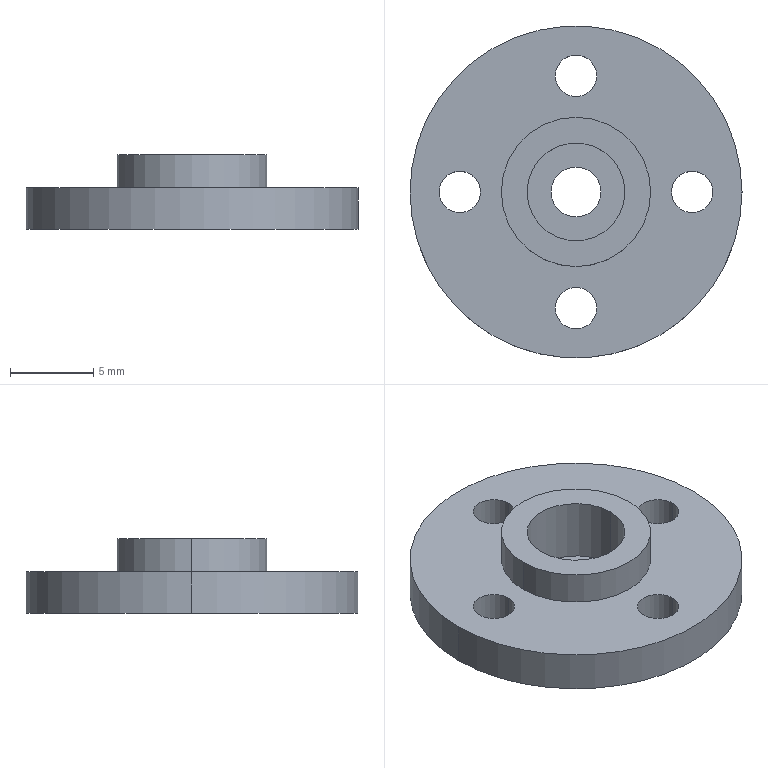Part | SolidWorks | features ICE 4, Extrusion 1, HoleWzd 1 | 1 solid | 20 faces | box 20 x 20 x 4.5 mm | volume 753.693 mm3 | cylinder 16 | plane 4 | commonest cylinder face diameters 2.5 x8 3 x2 5.9 x2 9 x2 20 x2
STEP:
#1=CARTESIAN_POINT('',(-8.25,0.,0.));
#2=VERTEX_POINT('',#1);
#3=CARTESIAN_POINT('',(-5.75,0.,0.));
#4=VERTEX_POINT('',#3);
#5=CARTESIAN_POINT('',(-7.,0.,0.));
#6=DIRECTION('',(0.,0.,1.));
#7=DIRECTION('',(1.,0.,0.));
#8=AXIS2_PLACEMENT_3D('',#5,#6,#7);
#9=CIRCLE('',#8,1.25);
#10=EDGE_CURVE('',#2,#4,#9,.T.);
#11=ORIENTED_EDGE('',*,*,#10,.F.);
#12=CARTESIAN_POINT('',(-8.25,0.,2.5));
#13=VERTEX_POINT('',#12);
#14=CARTESIAN_POINT('',(-8.25,0.,2.5));
#15=DIRECTION('',(0.,0.,1.));
#16=VECTOR('',#15,1000.);
#17=LINE('',#14,#16);
#18=EDGE_CURVE('',#2,#13,#17,.T.);
#19=ORIENTED_EDGE('',*,*,#18,.T.);
#20=CARTESIAN_POINT('',(-5.75,0.,2.5));
#21=VERTEX_POINT('',#20);
#22=CARTESIAN_POINT('',(-7.,0.,2.5));
#23=DIRECTION('',(0.,0.,1.));
#24=DIRECTION('',(1.,0.,0.));
#25=AXIS2_PLACEMENT_3D('',#22,#23,#24);
#26=CIRCLE('',#25,1.25);
#27=EDGE_CURVE('',#13,#21,#26,.T.);
#28=ORIENTED_EDGE('',*,*,#27,.T.);
#29=CARTESIAN_POINT('',(-5.75,0.,2.5));
#30=DIRECTION('',(0.,0.,1.));
#31=VECTOR('',#30,1000.);
#32=LINE('',#29,#31);
#33=EDGE_CURVE('',#4,#21,#32,.T.);
#34=ORIENTED_EDGE('',*,*,#33,.F.);
#35=EDGE_LOOP('',(#11,#19,#28,#34));
#36=FACE_OUTER_BOUND('',#35,.T.);
#37=CARTESIAN_POINT('',(-7.,0.,2.5));
#38=DIRECTION('',(0.,0.,1.));
#39=DIRECTION('',(1.,0.,0.));
#40=AXIS2_PLACEMENT_3D('',#37,#38,#39);
#41=CYLINDRICAL_SURFACE('',#40,1.25);
#42=ADVANCED_FACE('',(#36),#41,.F.);
#43=CARTESIAN_POINT('',(-1.25,7.,0.));
#44=VERTEX_POINT('',#43);
#45=CARTESIAN_POINT('',(1.25,7.,0.));
#46=VERTEX_POINT('',#45);
#47=CARTESIAN_POINT('',(0.,7.,0.));
#48=DIRECTION('',(0.,0.,1.));
#49=DIRECTION('',(1.,0.,0.));
#50=AXIS2_PLACEMENT_3D('',#47,#48,#49);
#51=CIRCLE('',#50,1.25);
#52=EDGE_CURVE('',#44,#46,#51,.T.);
#53=ORIENTED_EDGE('',*,*,#52,.F.);
#54=CARTESIAN_POINT('',(-1.25,7.,2.5));
#55=VERTEX_POINT('',#54);
#56=CARTESIAN_POINT('',(-1.25,7.,2.5));
#57=DIRECTION('',(0.,0.,1.));
#58=VECTOR('',#57,1000.);
#59=LINE('',#56,#58);
#60=EDGE_CURVE('',#44,#55,#59,.T.);
#61=ORIENTED_EDGE('',*,*,#60,.T.);
#62=CARTESIAN_POINT('',(1.25,7.,2.5));
#63=VERTEX_POINT('',#62);
#64=CARTESIAN_POINT('',(0.,7.,2.5));
#65=DIRECTION('',(0.,0.,1.));
#66=DIRECTION('',(1.,0.,0.));
#67=AXIS2_PLACEMENT_3D('',#64,#65,#66);
#68=CIRCLE('',#67,1.25);
#69=EDGE_CURVE('',#55,#63,#68,.T.);
#70=ORIENTED_EDGE('',*,*,#69,.T.);
#71=CARTESIAN_POINT('',(1.25,7.,2.5));
#72=DIRECTION('',(0.,0.,1.));
#73=VECTOR('',#72,1000.);
#74=LINE('',#71,#73);
#75=EDGE_CURVE('',#46,#63,#74,.T.);
#76=ORIENTED_EDGE('',*,*,#75,.F.);
#77=EDGE_LOOP('',(#53,#61,#70,#76));
#78=FACE_OUTER_BOUND('',#77,.T.);
#79=CARTESIAN_POINT('',(0.,7.,2.5));
#80=DIRECTION('',(0.,0.,1.));
#81=DIRECTION('',(1.,0.,0.));
#82=AXIS2_PLACEMENT_3D('',#79,#80,#81);
#83=CYLINDRICAL_SURFACE('',#82,1.25);
#84=ADVANCED_FACE('',(#78),#83,.F.);
#85=CARTESIAN_POINT('',(5.75,0.,0.));
#86=VERTEX_POINT('',#85);
#87=CARTESIAN_POINT('',(8.25,0.,0.));
#88=VERTEX_POINT('',#87);
#89=CARTESIAN_POINT('',(7.,0.,0.));
#90=DIRECTION('',(0.,0.,1.));
#91=DIRECTION('',(1.,0.,0.));
#92=AXIS2_PLACEMENT_3D('',#89,#90,#91);
#93=CIRCLE('',#92,1.25);
#94=EDGE_CURVE('',#86,#88,#93,.T.);
#95=ORIENTED_EDGE('',*,*,#94,.F.);
#96=CARTESIAN_POINT('',(5.75,0.,2.5));
#97=VERTEX_POINT('',#96);
#98=CARTESIAN_POINT('',(5.75,0.,2.5));
#99=DIRECTION('',(0.,0.,1.));
#100=VECTOR('',#99,1000.);
#101=LINE('',#98,#100);
#102=EDGE_CURVE('',#86,#97,#101,.T.);
#103=ORIENTED_EDGE('',*,*,#102,.T.);
#104=CARTESIAN_POINT('',(8.25,0.,2.5));
#105=VERTEX_POINT('',#104);
#106=CARTESIAN_POINT('',(7.,0.,2.5));
#107=DIRECTION('',(0.,0.,1.));
#108=DIRECTION('',(1.,0.,0.));
#109=AXIS2_PLACEMENT_3D('',#106,#107,#108);
#110=CIRCLE('',#109,1.25);
#111=EDGE_CURVE('',#97,#105,#110,.T.);
#112=ORIENTED_EDGE('',*,*,#111,.T.);
#113=CARTESIAN_POINT('',(8.25,0.,2.5));
#114=DIRECTION('',(0.,0.,1.));
#115=VECTOR('',#114,1000.);
#116=LINE('',#113,#115);
#117=EDGE_CURVE('',#88,#105,#116,.T.);
#118=ORIENTED_EDGE('',*,*,#117,.F.);
#119=EDGE_LOOP('',(#95,#103,#112,#118));
#120=FACE_OUTER_BOUND('',#119,.T.);
#121=CARTESIAN_POINT('',(7.,0.,2.5));
#122=DIRECTION('',(0.,0.,1.));
#123=DIRECTION('',(1.,0.,0.));
#124=AXIS2_PLACEMENT_3D('',#121,#122,#123);
#125=CYLINDRICAL_SURFACE('',#124,1.25);
#126=ADVANCED_FACE('',(#120),#125,.F.);
#127=CARTESIAN_POINT('',(-1.25,-7.,0.));
#128=VERTEX_POINT('',#127);
#129=CARTESIAN_POINT('',(1.25,-7.,0.));
#130=VERTEX_POINT('',#129);
#131=CARTESIAN_POINT('',(0.,-7.,0.));
#132=DIRECTION('',(0.,0.,1.));
#133=DIRECTION('',(1.,0.,0.));
#134=AXIS2_PLACEMENT_3D('',#131,#132,#133);
#135=CIRCLE('',#134,1.25);
#136=EDGE_CURVE('',#128,#130,#135,.T.);
#137=ORIENTED_EDGE('',*,*,#136,.F.);
#138=CARTESIAN_POINT('',(-1.25,-7.,2.5));
#139=VERTEX_POINT('',#138);
#140=CARTESIAN_POINT('',(-1.25,-7.,2.5));
#141=DIRECTION('',(0.,0.,1.));
#142=VECTOR('',#141,1000.);
#143=LINE('',#140,#142);
#144=EDGE_CURVE('',#128,#139,#143,.T.);
#145=ORIENTED_EDGE('',*,*,#144,.T.);
#146=CARTESIAN_POINT('',(1.25,-7.,2.5));
#147=VERTEX_POINT('',#146);
#148=CARTESIAN_POINT('',(0.,-7.,2.5));
#149=DIRECTION('',(0.,0.,1.));
#150=DIRECTION('',(1.,0.,0.));
#151=AXIS2_PLACEMENT_3D('',#148,#149,#150);
#152=CIRCLE('',#151,1.25);
#153=EDGE_CURVE('',#139,#147,#152,.T.);
#154=ORIENTED_EDGE('',*,*,#153,.T.);
#155=CARTESIAN_POINT('',(1.25,-7.,2.5));
#156=DIRECTION('',(0.,0.,1.));
#157=VECTOR('',#156,1000.);
#158=LINE('',#155,#157);
#159=EDGE_CURVE('',#130,#147,#158,.T.);
#160=ORIENTED_EDGE('',*,*,#159,.F.);
#161=EDGE_LOOP('',(#137,#145,#154,#160));
#162=FACE_OUTER_BOUND('',#161,.T.);
#163=CARTESIAN_POINT('',(0.,-7.,2.5));
#164=DIRECTION('',(0.,0.,1.));
#165=DIRECTION('',(1.,0.,0.));
#166=AXIS2_PLACEMENT_3D('',#163,#164,#165);
#167=CYLINDRICAL_SURFACE('',#166,1.25);
#168=ADVANCED_FACE('',(#162),#167,.F.);
#169=CARTESIAN_POINT('',(-1.5,0.,0.));
#170=VERTEX_POINT('',#169);
#171=CARTESIAN_POINT('',(1.5,0.,0.));
#172=VERTEX_POINT('',#171);
#173=CARTESIAN_POINT('',(0.,0.,0.));
#174=DIRECTION('',(0.,0.,1.));
#175=DIRECTION('',(1.,0.,0.));
#176=AXIS2_PLACEMENT_3D('',#173,#174,#175);
#177=CIRCLE('',#176,1.5);
#178=EDGE_CURVE('',#170,#172,#177,.T.);
#179=ORIENTED_EDGE('',*,*,#178,.F.);
#180=CARTESIAN_POINT('',(-1.5,0.,0.65));
#181=VERTEX_POINT('',#180);
#182=CARTESIAN_POINT('',(-1.5,0.,0.));
#183=DIRECTION('',(0.,0.,1.));
#184=VECTOR('',#183,1000.);
#185=LINE('',#182,#184);
#186=EDGE_CURVE('',#170,#181,#185,.T.);
#187=ORIENTED_EDGE('',*,*,#186,.T.);
#188=CARTESIAN_POINT('',(1.5,0.,0.65));
#189=VERTEX_POINT('',#188);
#190=CARTESIAN_POINT('',(0.,0.,0.65));
#191=DIRECTION('',(0.,0.,1.));
#192=DIRECTION('',(1.,0.,0.));
#193=AXIS2_PLACEMENT_3D('',#190,#191,#192);
#194=CIRCLE('',#193,1.5);
#195=EDGE_CURVE('',#181,#189,#194,.T.);
#196=ORIENTED_EDGE('',*,*,#195,.T.);
#197=CARTESIAN_POINT('',(1.5,0.,0.));
#198=DIRECTION('',(0.,0.,1.));
#199=VECTOR('',#198,1000.);
#200=LINE('',#197,#199);
#201=EDGE_CURVE('',#172,#189,#200,.T.);
#202=ORIENTED_EDGE('',*,*,#201,.F.);
#203=EDGE_LOOP('',(#179,#187,#196,#202));
#204=FACE_OUTER_BOUND('',#203,.T.);
#205=CARTESIAN_POINT('',(0.,0.,0.));
#206=DIRECTION('',(0.,0.,1.));
#207=DIRECTION('',(1.,0.,0.));
#208=AXIS2_PLACEMENT_3D('',#205,#206,#207);
#209=CYLINDRICAL_SURFACE('',#208,1.5);
#210=ADVANCED_FACE('',(#204),#209,.F.);
#211=CARTESIAN_POINT('',(-2.95,0.,0.65));
#212=VERTEX_POINT('',#211);
#213=CARTESIAN_POINT('',(2.95,0.,0.65));
#214=VERTEX_POINT('',#213);
#215=CARTESIAN_POINT('',(0.,0.,0.65));
#216=DIRECTION('',(0.,0.,1.));
#217=DIRECTION('',(1.,0.,0.));
#218=AXIS2_PLACEMENT_3D('',#215,#216,#217);
#219=CIRCLE('',#218,2.95);
#220=EDGE_CURVE('',#212,#214,#219,.T.);
#221=ORIENTED_EDGE('',*,*,#220,.F.);
#222=CARTESIAN_POINT('',(-2.95,0.,4.5));
#223=VERTEX_POINT('',#222);
#224=CARTESIAN_POINT('',(-2.95,0.,0.65));
#225=DIRECTION('',(0.,0.,1.));
#226=VECTOR('',#225,1000.);
#227=LINE('',#224,#226);
#228=EDGE_CURVE('',#212,#223,#227,.T.);
#229=ORIENTED_EDGE('',*,*,#228,.T.);
#230=CARTESIAN_POINT('',(2.95,0.,4.5));
#231=VERTEX_POINT('',#230);
#232=CARTESIAN_POINT('',(0.,0.,4.5));
#233=DIRECTION('',(0.,0.,1.));
#234=DIRECTION('',(1.,0.,0.));
#235=AXIS2_PLACEMENT_3D('',#232,#233,#234);
#236=CIRCLE('',#235,2.95);
#237=EDGE_CURVE('',#223,#231,#236,.T.);
#238=ORIENTED_EDGE('',*,*,#237,.T.);
#239=CARTESIAN_POINT('',(2.95,0.,0.65));
#240=DIRECTION('',(0.,0.,1.));
#241=VECTOR('',#240,1000.);
#242=LINE('',#239,#241);
#243=EDGE_CURVE('',#214,#231,#242,.T.);
#244=ORIENTED_EDGE('',*,*,#243,.F.);
#245=EDGE_LOOP('',(#221,#229,#238,#244));
#246=FACE_OUTER_BOUND('',#245,.T.);
#247=CARTESIAN_POINT('',(0.,0.,0.65));
#248=DIRECTION('',(0.,0.,1.));
#249=DIRECTION('',(1.,0.,0.));
#250=AXIS2_PLACEMENT_3D('',#247,#248,#249);
#251=CYLINDRICAL_SURFACE('',#250,2.95);
#252=ADVANCED_FACE('',(#246),#251,.F.);
#253=CARTESIAN_POINT('',(4.5,0.,2.5));
#254=VERTEX_POINT('',#253);
#255=CARTESIAN_POINT('',(-4.5,0.,2.5));
#256=VERTEX_POINT('',#255);
#257=CARTESIAN_POINT('',(0.,0.,2.5));
#258=DIRECTION('',(0.,0.,1.));
#259=DIRECTION('',(1.,0.,0.));
#260=AXIS2_PLACEMENT_3D('',#257,#258,#259);
#261=CIRCLE('',#260,4.5);
#262=EDGE_CURVE('',#254,#256,#261,.T.);
#263=ORIENTED_EDGE('',*,*,#262,.T.);
#264=CARTESIAN_POINT('',(-4.5,0.,4.5));
#265=VERTEX_POINT('',#264);
#266=CARTESIAN_POINT('',(-4.5,0.,2.5));
#267=DIRECTION('',(0.,0.,1.));
#268=VECTOR('',#267,1000.);
#269=LINE('',#266,#268);
#270=EDGE_CURVE('',#256,#265,#269,.T.);
#271=ORIENTED_EDGE('',*,*,#270,.T.);
#272=CARTESIAN_POINT('',(4.5,0.,4.5));
#273=VERTEX_POINT('',#272);
#274=CARTESIAN_POINT('',(0.,0.,4.5));
#275=DIRECTION('',(0.,0.,1.));
#276=DIRECTION('',(1.,0.,0.));
#277=AXIS2_PLACEMENT_3D('',#274,#275,#276);
#278=CIRCLE('',#277,4.5);
#279=EDGE_CURVE('',#273,#265,#278,.T.);
#280=ORIENTED_EDGE('',*,*,#279,.F.);
#281=CARTESIAN_POINT('',(4.5,0.,2.5));
#282=DIRECTION('',(0.,0.,1.));
#283=VECTOR('',#282,1000.);
#284=LINE('',#281,#283);
#285=EDGE_CURVE('',#254,#273,#284,.T.);
#286=ORIENTED_EDGE('',*,*,#285,.F.);
#287=EDGE_LOOP('',(#263,#271,#280,#286));
#288=FACE_OUTER_BOUND('',#287,.T.);
#289=CARTESIAN_POINT('',(0.,0.,2.5));
#290=DIRECTION('',(0.,0.,1.));
#291=DIRECTION('',(1.,0.,0.));
#292=AXIS2_PLACEMENT_3D('',#289,#290,#291);
#293=CYLINDRICAL_SURFACE('',#292,4.5);
#294=ADVANCED_FACE('',(#288),#293,.T.);
#295=CARTESIAN_POINT('',(10.,0.,2.5));
#296=VERTEX_POINT('',#295);
#297=CARTESIAN_POINT('',(-10.,0.,2.5));
#298=VERTEX_POINT('',#297);
#299=CARTESIAN_POINT('',(0.,0.,2.5));
#300=DIRECTION('',(0.,0.,1.));
#301=DIRECTION('',(1.,0.,0.));
#302=AXIS2_PLACEMENT_3D('',#299,#300,#301);
#303=CIRCLE('',#302,10.);
#304=EDGE_CURVE('',#296,#298,#303,.T.);
#305=ORIENTED_EDGE('',*,*,#304,.F.);
#306=CARTESIAN_POINT('',(10.,0.,0.));
#307=VERTEX_POINT('',#306);
#308=CARTESIAN_POINT('',(10.,0.,4.5));
#309=DIRECTION('',(0.,0.,-1.));
#310=VECTOR('',#309,1000.);
#311=LINE('',#308,#310);
#312=EDGE_CURVE('',#296,#307,#311,.T.);
#313=ORIENTED_EDGE('',*,*,#312,.T.);
#314=CARTESIAN_POINT('',(-10.,0.,0.));
#315=VERTEX_POINT('',#314);
#316=CARTESIAN_POINT('',(0.,0.,0.));
#317=DIRECTION('',(0.,0.,1.));
#318=DIRECTION('',(1.,0.,0.));
#319=AXIS2_PLACEMENT_3D('',#316,#317,#318);
#320=CIRCLE('',#319,10.);
#321=EDGE_CURVE('',#307,#315,#320,.T.);
#322=ORIENTED_EDGE('',*,*,#321,.T.);
#323=CARTESIAN_POINT('',(-10.,0.,4.5));
#324=DIRECTION('',(0.,0.,-1.));
#325=VECTOR('',#324,1000.);
#326=LINE('',#323,#325);
#327=EDGE_CURVE('',#298,#315,#326,.T.);
#328=ORIENTED_EDGE('',*,*,#327,.F.);
#329=EDGE_LOOP('',(#305,#313,#322,#328));
#330=FACE_OUTER_BOUND('',#329,.T.);
#331=CARTESIAN_POINT('',(0.,0.,4.5));
#332=DIRECTION('',(0.,0.,-1.));
#333=DIRECTION('',(-1.,0.,0.));
#334=AXIS2_PLACEMENT_3D('',#331,#332,#333);
#335=CYLINDRICAL_SURFACE('',#334,10.);
#336=ADVANCED_FACE('',(#330),#335,.T.);
#337=ORIENTED_EDGE('',*,*,#312,.F.);
#338=CARTESIAN_POINT('',(0.,0.,2.5));
#339=DIRECTION('',(0.,0.,1.));
#340=DIRECTION('',(1.,0.,0.));
#341=AXIS2_PLACEMENT_3D('',#338,#339,#340);
#342=CIRCLE('',#341,10.);
#343=EDGE_CURVE('',#298,#296,#342,.T.);
#344=ORIENTED_EDGE('',*,*,#343,.F.);
#345=ORIENTED_EDGE('',*,*,#327,.T.);
#346=CARTESIAN_POINT('',(0.,0.,0.));
#347=DIRECTION('',(0.,0.,1.));
#348=DIRECTION('',(1.,0.,0.));
#349=AXIS2_PLACEMENT_3D('',#346,#347,#348);
#350=CIRCLE('',#349,10.);
#351=EDGE_CURVE('',#315,#307,#350,.T.);
#352=ORIENTED_EDGE('',*,*,#351,.T.);
#353=EDGE_LOOP('',(#337,#344,#345,#352));
#354=FACE_OUTER_BOUND('',#353,.T.);
#355=CARTESIAN_POINT('',(0.,0.,4.5));
#356=DIRECTION('',(0.,0.,-1.));
#357=DIRECTION('',(-1.,0.,0.));
#358=AXIS2_PLACEMENT_3D('',#355,#356,#357);
#359=CYLINDRICAL_SURFACE('',#358,10.);
#360=ADVANCED_FACE('',(#354),#359,.T.);
#361=CARTESIAN_POINT('',(-7.,0.,0.));
#362=DIRECTION('',(0.,0.,1.));
#363=DIRECTION('',(1.,0.,0.));
#364=AXIS2_PLACEMENT_3D('',#361,#362,#363);
#365=CIRCLE('',#364,1.25);
#366=EDGE_CURVE('',#4,#2,#365,.T.);
#367=ORIENTED_EDGE('',*,*,#366,.T.);
#368=ORIENTED_EDGE('',*,*,#10,.T.);
#369=EDGE_LOOP('',(#367,#368));
#370=FACE_BOUND('',#369,.T.);
#371=CARTESIAN_POINT('',(0.,7.,0.));
#372=DIRECTION('',(0.,0.,1.));
#373=DIRECTION('',(1.,0.,0.));
#374=AXIS2_PLACEMENT_3D('',#371,#372,#373);
#375=CIRCLE('',#374,1.25);
#376=EDGE_CURVE('',#46,#44,#375,.T.);
#377=ORIENTED_EDGE('',*,*,#376,.T.);
#378=ORIENTED_EDGE('',*,*,#52,.T.);
#379=EDGE_LOOP('',(#377,#378));
#380=FACE_BOUND('',#379,.T.);
#381=CARTESIAN_POINT('',(7.,0.,0.));
#382=DIRECTION('',(0.,0.,1.));
#383=DIRECTION('',(1.,0.,0.));
#384=AXIS2_PLACEMENT_3D('',#381,#382,#383);
#385=CIRCLE('',#384,1.25);
#386=EDGE_CURVE('',#88,#86,#385,.T.);
#387=ORIENTED_EDGE('',*,*,#386,.T.);
#388=ORIENTED_EDGE('',*,*,#94,.T.);
#389=EDGE_LOOP('',(#387,#388));
#390=FACE_BOUND('',#389,.T.);
#391=CARTESIAN_POINT('',(0.,-7.,0.));
#392=DIRECTION('',(0.,0.,1.));
#393=DIRECTION('',(1.,0.,0.));
#394=AXIS2_PLACEMENT_3D('',#391,#392,#393);
#395=CIRCLE('',#394,1.25);
#396=EDGE_CURVE('',#130,#128,#395,.T.);
#397=ORIENTED_EDGE('',*,*,#396,.T.);
#398=ORIENTED_EDGE('',*,*,#136,.T.);
#399=EDGE_LOOP('',(#397,#398));
#400=FACE_BOUND('',#399,.T.);
#401=CARTESIAN_POINT('',(0.,0.,0.));
#402=DIRECTION('',(0.,0.,1.));
#403=DIRECTION('',(1.,0.,0.));
#404=AXIS2_PLACEMENT_3D('',#401,#402,#403);
#405=CIRCLE('',#404,1.5);
#406=EDGE_CURVE('',#172,#170,#405,.T.);
#407=ORIENTED_EDGE('',*,*,#406,.T.);
#408=ORIENTED_EDGE('',*,*,#178,.T.);
#409=EDGE_LOOP('',(#407,#408));
#410=FACE_BOUND('',#409,.T.);
#411=ORIENTED_EDGE('',*,*,#351,.F.);
#412=ORIENTED_EDGE('',*,*,#321,.F.);
#413=EDGE_LOOP('',(#411,#412));
#414=FACE_OUTER_BOUND('',#413,.T.);
#415=CARTESIAN_POINT('',(0.,0.,0.));
#416=DIRECTION('',(0.,0.,1.));
#417=DIRECTION('',(1.,0.,0.));
#418=AXIS2_PLACEMENT_3D('',#415,#416,#417);
#419=PLANE('',#418);
#420=ADVANCED_FACE('',(#370,#380,#390,#400,#410,#414),#419,.F.);
#421=CARTESIAN_POINT('',(-7.,0.,2.5));
#422=DIRECTION('',(0.,0.,1.));
#423=DIRECTION('',(1.,0.,0.));
#424=AXIS2_PLACEMENT_3D('',#421,#422,#423);
#425=CIRCLE('',#424,1.25);
#426=EDGE_CURVE('',#21,#13,#425,.T.);
#427=ORIENTED_EDGE('',*,*,#426,.F.);
#428=ORIENTED_EDGE('',*,*,#27,.F.);
#429=EDGE_LOOP('',(#427,#428));
#430=FACE_BOUND('',#429,.T.);
#431=CARTESIAN_POINT('',(0.,7.,2.5));
#432=DIRECTION('',(0.,0.,1.));
#433=DIRECTION('',(1.,0.,0.));
#434=AXIS2_PLACEMENT_3D('',#431,#432,#433);
#435=CIRCLE('',#434,1.25);
#436=EDGE_CURVE('',#63,#55,#435,.T.);
#437=ORIENTED_EDGE('',*,*,#436,.F.);
#438=ORIENTED_EDGE('',*,*,#69,.F.);
#439=EDGE_LOOP('',(#437,#438));
#440=FACE_BOUND('',#439,.T.);
#441=CARTESIAN_POINT('',(7.,0.,2.5));
#442=DIRECTION('',(0.,0.,1.));
#443=DIRECTION('',(1.,0.,0.));
#444=AXIS2_PLACEMENT_3D('',#441,#442,#443);
#445=CIRCLE('',#444,1.25);
#446=EDGE_CURVE('',#105,#97,#445,.T.);
#447=ORIENTED_EDGE('',*,*,#446,.F.);
#448=ORIENTED_EDGE('',*,*,#111,.F.);
#449=EDGE_LOOP('',(#447,#448));
#450=FACE_BOUND('',#449,.T.);
#451=CARTESIAN_POINT('',(0.,-7.,2.5));
#452=DIRECTION('',(0.,0.,1.));
#453=DIRECTION('',(1.,0.,0.));
#454=AXIS2_PLACEMENT_3D('',#451,#452,#453);
#455=CIRCLE('',#454,1.25);
#456=EDGE_CURVE('',#147,#139,#455,.T.);
#457=ORIENTED_EDGE('',*,*,#456,.F.);
#458=ORIENTED_EDGE('',*,*,#153,.F.);
#459=EDGE_LOOP('',(#457,#458));
#460=FACE_BOUND('',#459,.T.);
#461=ORIENTED_EDGE('',*,*,#262,.F.);
#462=CARTESIAN_POINT('',(0.,0.,2.5));
#463=DIRECTION('',(0.,0.,1.));
#464=DIRECTION('',(1.,0.,0.));
#465=AXIS2_PLACEMENT_3D('',#462,#463,#464);
#466=CIRCLE('',#465,4.5);
#467=EDGE_CURVE('',#256,#254,#466,.T.);
#468=ORIENTED_EDGE('',*,*,#467,.F.);
#469=EDGE_LOOP('',(#461,#468));
#470=FACE_BOUND('',#469,.T.);
#471=ORIENTED_EDGE('',*,*,#343,.T.);
#472=ORIENTED_EDGE('',*,*,#304,.T.);
#473=EDGE_LOOP('',(#471,#472));
#474=FACE_OUTER_BOUND('',#473,.T.);
#475=CARTESIAN_POINT('',(0.,0.,2.5));
#476=DIRECTION('',(0.,0.,1.));
#477=DIRECTION('',(1.,0.,0.));
#478=AXIS2_PLACEMENT_3D('',#475,#476,#477);
#479=PLANE('',#478);
#480=ADVANCED_FACE('',(#430,#440,#450,#460,#470,#474),#479,.T.);
#481=ORIENTED_EDGE('',*,*,#270,.F.);
#482=ORIENTED_EDGE('',*,*,#467,.T.);
#483=ORIENTED_EDGE('',*,*,#285,.T.);
#484=CARTESIAN_POINT('',(0.,0.,4.5));
#485=DIRECTION('',(0.,0.,1.));
#486=DIRECTION('',(1.,0.,0.));
#487=AXIS2_PLACEMENT_3D('',#484,#485,#486);
#488=CIRCLE('',#487,4.5);
#489=EDGE_CURVE('',#265,#273,#488,.T.);
#490=ORIENTED_EDGE('',*,*,#489,.F.);
#491=EDGE_LOOP('',(#481,#482,#483,#490));
#492=FACE_OUTER_BOUND('',#491,.T.);
#493=CARTESIAN_POINT('',(0.,0.,2.5));
#494=DIRECTION('',(0.,0.,1.));
#495=DIRECTION('',(1.,0.,0.));
#496=AXIS2_PLACEMENT_3D('',#493,#494,#495);
#497=CYLINDRICAL_SURFACE('',#496,4.5);
#498=ADVANCED_FACE('',(#492),#497,.T.);
#499=CARTESIAN_POINT('',(0.,0.,4.5));
#500=DIRECTION('',(0.,0.,1.));
#501=DIRECTION('',(1.,0.,0.));
#502=AXIS2_PLACEMENT_3D('',#499,#500,#501);
#503=CIRCLE('',#502,2.95);
#504=EDGE_CURVE('',#231,#223,#503,.T.);
#505=ORIENTED_EDGE('',*,*,#504,.F.);
#506=ORIENTED_EDGE('',*,*,#237,.F.);
#507=EDGE_LOOP('',(#505,#506));
#508=FACE_BOUND('',#507,.T.);
#509=ORIENTED_EDGE('',*,*,#279,.T.);
#510=ORIENTED_EDGE('',*,*,#489,.T.);
#511=EDGE_LOOP('',(#509,#510));
#512=FACE_OUTER_BOUND('',#511,.T.);
#513=CARTESIAN_POINT('',(0.,0.,4.5));
#514=DIRECTION('',(0.,0.,1.));
#515=DIRECTION('',(1.,0.,0.));
#516=AXIS2_PLACEMENT_3D('',#513,#514,#515);
#517=PLANE('',#516);
#518=ADVANCED_FACE('',(#508,#512),#517,.T.);
#519=ORIENTED_EDGE('',*,*,#228,.F.);
#520=CARTESIAN_POINT('',(0.,0.,0.65));
#521=DIRECTION('',(0.,0.,1.));
#522=DIRECTION('',(1.,0.,0.));
#523=AXIS2_PLACEMENT_3D('',#520,#521,#522);
#524=CIRCLE('',#523,2.95);
#525=EDGE_CURVE('',#214,#212,#524,.T.);
#526=ORIENTED_EDGE('',*,*,#525,.F.);
#527=ORIENTED_EDGE('',*,*,#243,.T.);
#528=ORIENTED_EDGE('',*,*,#504,.T.);
#529=EDGE_LOOP('',(#519,#526,#527,#528));
#530=FACE_OUTER_BOUND('',#529,.T.);
#531=CARTESIAN_POINT('',(0.,0.,0.65));
#532=DIRECTION('',(0.,0.,1.));
#533=DIRECTION('',(1.,0.,0.));
#534=AXIS2_PLACEMENT_3D('',#531,#532,#533);
#535=CYLINDRICAL_SURFACE('',#534,2.95);
#536=ADVANCED_FACE('',(#530),#535,.F.);
#537=CARTESIAN_POINT('',(0.,0.,0.65));
#538=DIRECTION('',(0.,0.,1.));
#539=DIRECTION('',(1.,0.,0.));
#540=AXIS2_PLACEMENT_3D('',#537,#538,#539);
#541=CIRCLE('',#540,1.5);
#542=EDGE_CURVE('',#189,#181,#541,.T.);
#543=ORIENTED_EDGE('',*,*,#542,.F.);
#544=ORIENTED_EDGE('',*,*,#195,.F.);
#545=EDGE_LOOP('',(#543,#544));
#546=FACE_BOUND('',#545,.T.);
#547=ORIENTED_EDGE('',*,*,#525,.T.);
#548=ORIENTED_EDGE('',*,*,#220,.T.);
#549=EDGE_LOOP('',(#547,#548));
#550=FACE_OUTER_BOUND('',#549,.T.);
#551=CARTESIAN_POINT('',(0.,0.,0.65));
#552=DIRECTION('',(0.,0.,1.));
#553=DIRECTION('',(1.,0.,0.));
#554=AXIS2_PLACEMENT_3D('',#551,#552,#553);
#555=PLANE('',#554);
#556=ADVANCED_FACE('',(#546,#550),#555,.T.);
#557=ORIENTED_EDGE('',*,*,#186,.F.);
#558=ORIENTED_EDGE('',*,*,#406,.F.);
#559=ORIENTED_EDGE('',*,*,#201,.T.);
#560=ORIENTED_EDGE('',*,*,#542,.T.);
#561=EDGE_LOOP('',(#557,#558,#559,#560));
#562=FACE_OUTER_BOUND('',#561,.T.);
#563=CARTESIAN_POINT('',(0.,0.,0.));
#564=DIRECTION('',(0.,0.,1.));
#565=DIRECTION('',(1.,0.,0.));
#566=AXIS2_PLACEMENT_3D('',#563,#564,#565);
#567=CYLINDRICAL_SURFACE('',#566,1.5);
#568=ADVANCED_FACE('',(#562),#567,.F.);
#569=ORIENTED_EDGE('',*,*,#144,.F.);
#570=ORIENTED_EDGE('',*,*,#396,.F.);
#571=ORIENTED_EDGE('',*,*,#159,.T.);
#572=ORIENTED_EDGE('',*,*,#456,.T.);
#573=EDGE_LOOP('',(#569,#570,#571,#572));
#574=FACE_OUTER_BOUND('',#573,.T.);
#575=CARTESIAN_POINT('',(0.,-7.,2.5));
#576=DIRECTION('',(0.,0.,1.));
#577=DIRECTION('',(1.,0.,0.));
#578=AXIS2_PLACEMENT_3D('',#575,#576,#577);
#579=CYLINDRICAL_SURFACE('',#578,1.25);
#580=ADVANCED_FACE('',(#574),#579,.F.);
#581=ORIENTED_EDGE('',*,*,#102,.F.);
#582=ORIENTED_EDGE('',*,*,#386,.F.);
#583=ORIENTED_EDGE('',*,*,#117,.T.);
#584=ORIENTED_EDGE('',*,*,#446,.T.);
#585=EDGE_LOOP('',(#581,#582,#583,#584));
#586=FACE_OUTER_BOUND('',#585,.T.);
#587=CARTESIAN_POINT('',(7.,0.,2.5));
#588=DIRECTION('',(0.,0.,1.));
#589=DIRECTION('',(1.,0.,0.));
#590=AXIS2_PLACEMENT_3D('',#587,#588,#589);
#591=CYLINDRICAL_SURFACE('',#590,1.25);
#592=ADVANCED_FACE('',(#586),#591,.F.);
#593=ORIENTED_EDGE('',*,*,#60,.F.);
#594=ORIENTED_EDGE('',*,*,#376,.F.);
#595=ORIENTED_EDGE('',*,*,#75,.T.);
#596=ORIENTED_EDGE('',*,*,#436,.T.);
#597=EDGE_LOOP('',(#593,#594,#595,#596));
#598=FACE_OUTER_BOUND('',#597,.T.);
#599=CARTESIAN_POINT('',(0.,7.,2.5));
#600=DIRECTION('',(0.,0.,1.));
#601=DIRECTION('',(1.,0.,0.));
#602=AXIS2_PLACEMENT_3D('',#599,#600,#601);
#603=CYLINDRICAL_SURFACE('',#602,1.25);
#604=ADVANCED_FACE('',(#598),#603,.F.);
#605=ORIENTED_EDGE('',*,*,#18,.F.);
#606=ORIENTED_EDGE('',*,*,#366,.F.);
#607=ORIENTED_EDGE('',*,*,#33,.T.);
#608=ORIENTED_EDGE('',*,*,#426,.T.);
#609=EDGE_LOOP('',(#605,#606,#607,#608));
#610=FACE_OUTER_BOUND('',#609,.T.);
#611=CARTESIAN_POINT('',(-7.,0.,2.5));
#612=DIRECTION('',(0.,0.,1.));
#613=DIRECTION('',(1.,0.,0.));
#614=AXIS2_PLACEMENT_3D('',#611,#612,#613);
#615=CYLINDRICAL_SURFACE('',#614,1.25);
#616=ADVANCED_FACE('',(#610),#615,.F.);
#617=CLOSED_SHELL('',(#42,#84,#126,#168,#210,#252,#294,#336,#360,#420,#480,#498,#518,#536,#556,#568,#580,#592,#604,#616));
#618=MANIFOLD_SOLID_BREP('',#617);
#619=CARTESIAN_POINT('',(0.,0.,0.));
#620=DIRECTION('',(0.,0.,1.));
#621=DIRECTION('',(1.,0.,0.));
#622=AXIS2_PLACEMENT_3D('',#619,#620,#621);
#623=(LENGTH_UNIT()NAMED_UNIT(*)SI_UNIT(.MILLI.,.METRE.));
#624=UNCERTAINTY_MEASURE_WITH_UNIT(LENGTH_MEASURE(0.00001),#623,'','');
#625=(NAMED_UNIT(*)PLANE_ANGLE_UNIT()SI_UNIT($,.RADIAN.));
#626=(NAMED_UNIT(*)SI_UNIT($,.STERADIAN.)SOLID_ANGLE_UNIT());
#627=(GEOMETRIC_REPRESENTATION_CONTEXT(3)GLOBAL_UNCERTAINTY_ASSIGNED_CONTEXT((#624))GLOBAL_UNIT_ASSIGNED_CONTEXT((#623,#625,#626))REPRESENTATION_CONTEXT('',''));
#628=ADVANCED_BREP_SHAPE_REPRESENTATION('',(#618,#622),#627);